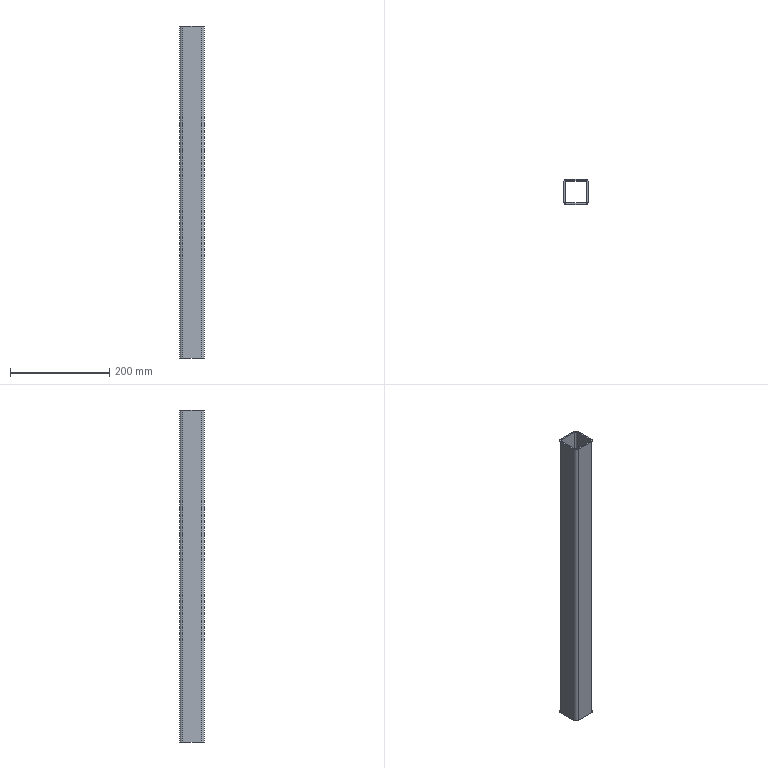Part | SolidWorks | 1 solid | 18 faces | box 50 x 50 x 670 mm | volume 362351 mm3 | plane 10 | cylinder 8 | commonest cylinder face diameters 6 x4 12 x4
STEP:
#1=CARTESIAN_POINT('',(19.,25.,335.));
#2=VERTEX_POINT('',#1);
#3=CARTESIAN_POINT('',(25.,19.,335.));
#4=VERTEX_POINT('',#3);
#5=CARTESIAN_POINT('',(19.,19.,335.));
#6=DIRECTION('',(0.,0.,-1.));
#7=DIRECTION('',(-1.,0.,0.));
#8=AXIS2_PLACEMENT_3D('',#5,#6,#7);
#9=CIRCLE('',#8,6.);
#10=EDGE_CURVE('',#2,#4,#9,.T.);
#11=ORIENTED_EDGE('',*,*,#10,.T.);
#12=CARTESIAN_POINT('',(25.,19.,-335.));
#13=VERTEX_POINT('',#12);
#14=CARTESIAN_POINT('',(25.,19.,-335.));
#15=DIRECTION('',(0.,0.,1.));
#16=VECTOR('',#15,1000.);
#17=LINE('',#14,#16);
#18=EDGE_CURVE('',#13,#4,#17,.T.);
#19=ORIENTED_EDGE('',*,*,#18,.F.);
#20=CARTESIAN_POINT('',(19.,25.,-335.));
#21=VERTEX_POINT('',#20);
#22=CARTESIAN_POINT('',(19.,19.,-335.));
#23=DIRECTION('',(0.,0.,-1.));
#24=DIRECTION('',(-1.,0.,0.));
#25=AXIS2_PLACEMENT_3D('',#22,#23,#24);
#26=CIRCLE('',#25,6.);
#27=EDGE_CURVE('',#21,#13,#26,.T.);
#28=ORIENTED_EDGE('',*,*,#27,.F.);
#29=CARTESIAN_POINT('',(19.,25.,-335.));
#30=DIRECTION('',(0.,0.,1.));
#31=VECTOR('',#30,1000.);
#32=LINE('',#29,#31);
#33=EDGE_CURVE('',#21,#2,#32,.T.);
#34=ORIENTED_EDGE('',*,*,#33,.T.);
#35=EDGE_LOOP('',(#11,#19,#28,#34));
#36=FACE_OUTER_BOUND('',#35,.T.);
#37=CARTESIAN_POINT('',(19.,19.,-335.));
#38=DIRECTION('',(0.,0.,1.));
#39=DIRECTION('',(1.,0.,0.));
#40=AXIS2_PLACEMENT_3D('',#37,#38,#39);
#41=CYLINDRICAL_SURFACE('',#40,6.);
#42=ADVANCED_FACE('',(#36),#41,.T.);
#43=CARTESIAN_POINT('',(25.,-19.,335.));
#44=VERTEX_POINT('',#43);
#45=CARTESIAN_POINT('',(25.,19.,335.));
#46=DIRECTION('',(0.,-1.,0.));
#47=VECTOR('',#46,1000.);
#48=LINE('',#45,#47);
#49=EDGE_CURVE('',#4,#44,#48,.T.);
#50=ORIENTED_EDGE('',*,*,#49,.T.);
#51=CARTESIAN_POINT('',(25.,-19.,-335.));
#52=VERTEX_POINT('',#51);
#53=CARTESIAN_POINT('',(25.,-19.,-335.));
#54=DIRECTION('',(0.,0.,1.));
#55=VECTOR('',#54,1000.);
#56=LINE('',#53,#55);
#57=EDGE_CURVE('',#52,#44,#56,.T.);
#58=ORIENTED_EDGE('',*,*,#57,.F.);
#59=CARTESIAN_POINT('',(25.,19.,-335.));
#60=DIRECTION('',(0.,-1.,0.));
#61=VECTOR('',#60,1000.);
#62=LINE('',#59,#61);
#63=EDGE_CURVE('',#13,#52,#62,.T.);
#64=ORIENTED_EDGE('',*,*,#63,.F.);
#65=ORIENTED_EDGE('',*,*,#18,.T.);
#66=EDGE_LOOP('',(#50,#58,#64,#65));
#67=FACE_OUTER_BOUND('',#66,.T.);
#68=CARTESIAN_POINT('',(25.,19.,-335.));
#69=DIRECTION('',(-1.,0.,0.));
#70=DIRECTION('',(0.,0.,1.));
#71=AXIS2_PLACEMENT_3D('',#68,#69,#70);
#72=PLANE('',#71);
#73=ADVANCED_FACE('',(#67),#72,.F.);
#74=CARTESIAN_POINT('',(19.,-25.,335.));
#75=VERTEX_POINT('',#74);
#76=CARTESIAN_POINT('',(19.,-19.,335.));
#77=DIRECTION('',(0.,0.,-1.));
#78=DIRECTION('',(-1.,0.,0.));
#79=AXIS2_PLACEMENT_3D('',#76,#77,#78);
#80=CIRCLE('',#79,6.);
#81=EDGE_CURVE('',#44,#75,#80,.T.);
#82=ORIENTED_EDGE('',*,*,#81,.T.);
#83=CARTESIAN_POINT('',(19.,-25.,-335.));
#84=VERTEX_POINT('',#83);
#85=CARTESIAN_POINT('',(19.,-25.,-335.));
#86=DIRECTION('',(0.,0.,1.));
#87=VECTOR('',#86,1000.);
#88=LINE('',#85,#87);
#89=EDGE_CURVE('',#84,#75,#88,.T.);
#90=ORIENTED_EDGE('',*,*,#89,.F.);
#91=CARTESIAN_POINT('',(19.,-19.,-335.));
#92=DIRECTION('',(0.,0.,-1.));
#93=DIRECTION('',(-1.,0.,0.));
#94=AXIS2_PLACEMENT_3D('',#91,#92,#93);
#95=CIRCLE('',#94,6.);
#96=EDGE_CURVE('',#52,#84,#95,.T.);
#97=ORIENTED_EDGE('',*,*,#96,.F.);
#98=ORIENTED_EDGE('',*,*,#57,.T.);
#99=EDGE_LOOP('',(#82,#90,#97,#98));
#100=FACE_OUTER_BOUND('',#99,.T.);
#101=CARTESIAN_POINT('',(19.,-19.,-335.));
#102=DIRECTION('',(0.,0.,1.));
#103=DIRECTION('',(1.,0.,0.));
#104=AXIS2_PLACEMENT_3D('',#101,#102,#103);
#105=CYLINDRICAL_SURFACE('',#104,6.);
#106=ADVANCED_FACE('',(#100),#105,.T.);
#107=CARTESIAN_POINT('',(-19.,-25.,335.));
#108=VERTEX_POINT('',#107);
#109=CARTESIAN_POINT('',(-19.,-25.,335.));
#110=DIRECTION('',(-1.,0.,0.));
#111=VECTOR('',#110,1000.);
#112=LINE('',#109,#111);
#113=EDGE_CURVE('',#75,#108,#112,.T.);
#114=ORIENTED_EDGE('',*,*,#113,.T.);
#115=CARTESIAN_POINT('',(-19.,-25.,-335.));
#116=VERTEX_POINT('',#115);
#117=CARTESIAN_POINT('',(-19.,-25.,-335.));
#118=DIRECTION('',(0.,0.,1.));
#119=VECTOR('',#118,1000.);
#120=LINE('',#117,#119);
#121=EDGE_CURVE('',#116,#108,#120,.T.);
#122=ORIENTED_EDGE('',*,*,#121,.F.);
#123=CARTESIAN_POINT('',(-19.,-25.,-335.));
#124=DIRECTION('',(-1.,0.,0.));
#125=VECTOR('',#124,1000.);
#126=LINE('',#123,#125);
#127=EDGE_CURVE('',#84,#116,#126,.T.);
#128=ORIENTED_EDGE('',*,*,#127,.F.);
#129=ORIENTED_EDGE('',*,*,#89,.T.);
#130=EDGE_LOOP('',(#114,#122,#128,#129));
#131=FACE_OUTER_BOUND('',#130,.T.);
#132=CARTESIAN_POINT('',(-19.,-25.,-335.));
#133=DIRECTION('',(0.,1.,0.));
#134=DIRECTION('',(0.,0.,1.));
#135=AXIS2_PLACEMENT_3D('',#132,#133,#134);
#136=PLANE('',#135);
#137=ADVANCED_FACE('',(#131),#136,.F.);
#138=CARTESIAN_POINT('',(-25.,-19.,335.));
#139=VERTEX_POINT('',#138);
#140=CARTESIAN_POINT('',(-19.,-19.,335.));
#141=DIRECTION('',(0.,0.,-1.));
#142=DIRECTION('',(-1.,0.,0.));
#143=AXIS2_PLACEMENT_3D('',#140,#141,#142);
#144=CIRCLE('',#143,6.);
#145=EDGE_CURVE('',#108,#139,#144,.T.);
#146=ORIENTED_EDGE('',*,*,#145,.T.);
#147=CARTESIAN_POINT('',(-25.,-19.,-335.));
#148=VERTEX_POINT('',#147);
#149=CARTESIAN_POINT('',(-25.,-19.,-335.));
#150=DIRECTION('',(0.,0.,1.));
#151=VECTOR('',#150,1000.);
#152=LINE('',#149,#151);
#153=EDGE_CURVE('',#148,#139,#152,.T.);
#154=ORIENTED_EDGE('',*,*,#153,.F.);
#155=CARTESIAN_POINT('',(-19.,-19.,-335.));
#156=DIRECTION('',(0.,0.,-1.));
#157=DIRECTION('',(-1.,0.,0.));
#158=AXIS2_PLACEMENT_3D('',#155,#156,#157);
#159=CIRCLE('',#158,6.);
#160=EDGE_CURVE('',#116,#148,#159,.T.);
#161=ORIENTED_EDGE('',*,*,#160,.F.);
#162=ORIENTED_EDGE('',*,*,#121,.T.);
#163=EDGE_LOOP('',(#146,#154,#161,#162));
#164=FACE_OUTER_BOUND('',#163,.T.);
#165=CARTESIAN_POINT('',(-19.,-19.,-335.));
#166=DIRECTION('',(0.,0.,1.));
#167=DIRECTION('',(1.,0.,0.));
#168=AXIS2_PLACEMENT_3D('',#165,#166,#167);
#169=CYLINDRICAL_SURFACE('',#168,6.);
#170=ADVANCED_FACE('',(#164),#169,.T.);
#171=CARTESIAN_POINT('',(-25.,19.,335.));
#172=VERTEX_POINT('',#171);
#173=CARTESIAN_POINT('',(-25.,-19.,335.));
#174=DIRECTION('',(0.,1.,0.));
#175=VECTOR('',#174,1000.);
#176=LINE('',#173,#175);
#177=EDGE_CURVE('',#139,#172,#176,.T.);
#178=ORIENTED_EDGE('',*,*,#177,.T.);
#179=CARTESIAN_POINT('',(-25.,19.,-335.));
#180=VERTEX_POINT('',#179);
#181=CARTESIAN_POINT('',(-25.,19.,-335.));
#182=DIRECTION('',(0.,0.,1.));
#183=VECTOR('',#182,1000.);
#184=LINE('',#181,#183);
#185=EDGE_CURVE('',#180,#172,#184,.T.);
#186=ORIENTED_EDGE('',*,*,#185,.F.);
#187=CARTESIAN_POINT('',(-25.,-19.,-335.));
#188=DIRECTION('',(0.,1.,0.));
#189=VECTOR('',#188,1000.);
#190=LINE('',#187,#189);
#191=EDGE_CURVE('',#148,#180,#190,.T.);
#192=ORIENTED_EDGE('',*,*,#191,.F.);
#193=ORIENTED_EDGE('',*,*,#153,.T.);
#194=EDGE_LOOP('',(#178,#186,#192,#193));
#195=FACE_OUTER_BOUND('',#194,.T.);
#196=CARTESIAN_POINT('',(-25.,-19.,-335.));
#197=DIRECTION('',(1.,0.,0.));
#198=DIRECTION('',(0.,0.,-1.));
#199=AXIS2_PLACEMENT_3D('',#196,#197,#198);
#200=PLANE('',#199);
#201=ADVANCED_FACE('',(#195),#200,.F.);
#202=CARTESIAN_POINT('',(-19.,25.,335.));
#203=VERTEX_POINT('',#202);
#204=CARTESIAN_POINT('',(-19.,19.,335.));
#205=DIRECTION('',(0.,0.,-1.));
#206=DIRECTION('',(-1.,0.,0.));
#207=AXIS2_PLACEMENT_3D('',#204,#205,#206);
#208=CIRCLE('',#207,6.);
#209=EDGE_CURVE('',#172,#203,#208,.T.);
#210=ORIENTED_EDGE('',*,*,#209,.T.);
#211=CARTESIAN_POINT('',(-19.,25.,-335.));
#212=VERTEX_POINT('',#211);
#213=CARTESIAN_POINT('',(-19.,25.,-335.));
#214=DIRECTION('',(0.,0.,1.));
#215=VECTOR('',#214,1000.);
#216=LINE('',#213,#215);
#217=EDGE_CURVE('',#212,#203,#216,.T.);
#218=ORIENTED_EDGE('',*,*,#217,.F.);
#219=CARTESIAN_POINT('',(-19.,19.,-335.));
#220=DIRECTION('',(0.,0.,-1.));
#221=DIRECTION('',(-1.,0.,0.));
#222=AXIS2_PLACEMENT_3D('',#219,#220,#221);
#223=CIRCLE('',#222,6.);
#224=EDGE_CURVE('',#180,#212,#223,.T.);
#225=ORIENTED_EDGE('',*,*,#224,.F.);
#226=ORIENTED_EDGE('',*,*,#185,.T.);
#227=EDGE_LOOP('',(#210,#218,#225,#226));
#228=FACE_OUTER_BOUND('',#227,.T.);
#229=CARTESIAN_POINT('',(-19.,19.,-335.));
#230=DIRECTION('',(0.,0.,1.));
#231=DIRECTION('',(1.,0.,0.));
#232=AXIS2_PLACEMENT_3D('',#229,#230,#231);
#233=CYLINDRICAL_SURFACE('',#232,6.);
#234=ADVANCED_FACE('',(#228),#233,.T.);
#235=CARTESIAN_POINT('',(22.,-19.,335.));
#236=VERTEX_POINT('',#235);
#237=CARTESIAN_POINT('',(19.,-22.,335.));
#238=VERTEX_POINT('',#237);
#239=CARTESIAN_POINT('',(19.,-19.,335.));
#240=DIRECTION('',(0.,0.,-1.));
#241=DIRECTION('',(-1.,0.,0.));
#242=AXIS2_PLACEMENT_3D('',#239,#240,#241);
#243=CIRCLE('',#242,3.);
#244=EDGE_CURVE('',#236,#238,#243,.T.);
#245=ORIENTED_EDGE('',*,*,#244,.F.);
#246=CARTESIAN_POINT('',(22.,-19.,-335.));
#247=VERTEX_POINT('',#246);
#248=CARTESIAN_POINT('',(22.,-19.,-335.));
#249=DIRECTION('',(0.,0.,1.));
#250=VECTOR('',#249,1000.);
#251=LINE('',#248,#250);
#252=EDGE_CURVE('',#247,#236,#251,.T.);
#253=ORIENTED_EDGE('',*,*,#252,.F.);
#254=CARTESIAN_POINT('',(19.,-22.,-335.));
#255=VERTEX_POINT('',#254);
#256=CARTESIAN_POINT('',(19.,-19.,-335.));
#257=DIRECTION('',(0.,0.,-1.));
#258=DIRECTION('',(-1.,0.,0.));
#259=AXIS2_PLACEMENT_3D('',#256,#257,#258);
#260=CIRCLE('',#259,3.);
#261=EDGE_CURVE('',#247,#255,#260,.T.);
#262=ORIENTED_EDGE('',*,*,#261,.T.);
#263=CARTESIAN_POINT('',(19.,-22.,-335.));
#264=DIRECTION('',(0.,0.,1.));
#265=VECTOR('',#264,1000.);
#266=LINE('',#263,#265);
#267=EDGE_CURVE('',#255,#238,#266,.T.);
#268=ORIENTED_EDGE('',*,*,#267,.T.);
#269=EDGE_LOOP('',(#245,#253,#262,#268));
#270=FACE_OUTER_BOUND('',#269,.T.);
#271=CARTESIAN_POINT('',(19.,-19.,-335.));
#272=DIRECTION('',(0.,0.,1.));
#273=DIRECTION('',(1.,0.,0.));
#274=AXIS2_PLACEMENT_3D('',#271,#272,#273);
#275=CYLINDRICAL_SURFACE('',#274,3.);
#276=ADVANCED_FACE('',(#270),#275,.F.);
#277=CARTESIAN_POINT('',(22.,19.,335.));
#278=VERTEX_POINT('',#277);
#279=CARTESIAN_POINT('',(22.,19.,335.));
#280=DIRECTION('',(0.,-1.,0.));
#281=VECTOR('',#280,1000.);
#282=LINE('',#279,#281);
#283=EDGE_CURVE('',#278,#236,#282,.T.);
#284=ORIENTED_EDGE('',*,*,#283,.F.);
#285=CARTESIAN_POINT('',(22.,19.,-335.));
#286=VERTEX_POINT('',#285);
#287=CARTESIAN_POINT('',(22.,19.,-335.));
#288=DIRECTION('',(0.,0.,1.));
#289=VECTOR('',#288,1000.);
#290=LINE('',#287,#289);
#291=EDGE_CURVE('',#286,#278,#290,.T.);
#292=ORIENTED_EDGE('',*,*,#291,.F.);
#293=CARTESIAN_POINT('',(22.,19.,-335.));
#294=DIRECTION('',(0.,-1.,0.));
#295=VECTOR('',#294,1000.);
#296=LINE('',#293,#295);
#297=EDGE_CURVE('',#286,#247,#296,.T.);
#298=ORIENTED_EDGE('',*,*,#297,.T.);
#299=ORIENTED_EDGE('',*,*,#252,.T.);
#300=EDGE_LOOP('',(#284,#292,#298,#299));
#301=FACE_OUTER_BOUND('',#300,.T.);
#302=CARTESIAN_POINT('',(22.,19.,-335.));
#303=DIRECTION('',(-1.,0.,0.));
#304=DIRECTION('',(0.,0.,1.));
#305=AXIS2_PLACEMENT_3D('',#302,#303,#304);
#306=PLANE('',#305);
#307=ADVANCED_FACE('',(#301),#306,.T.);
#308=CARTESIAN_POINT('',(19.,22.,335.));
#309=VERTEX_POINT('',#308);
#310=CARTESIAN_POINT('',(19.,19.,335.));
#311=DIRECTION('',(0.,0.,-1.));
#312=DIRECTION('',(-1.,0.,0.));
#313=AXIS2_PLACEMENT_3D('',#310,#311,#312);
#314=CIRCLE('',#313,3.);
#315=EDGE_CURVE('',#309,#278,#314,.T.);
#316=ORIENTED_EDGE('',*,*,#315,.F.);
#317=CARTESIAN_POINT('',(19.,22.,-335.));
#318=VERTEX_POINT('',#317);
#319=CARTESIAN_POINT('',(19.,22.,-335.));
#320=DIRECTION('',(0.,0.,1.));
#321=VECTOR('',#320,1000.);
#322=LINE('',#319,#321);
#323=EDGE_CURVE('',#318,#309,#322,.T.);
#324=ORIENTED_EDGE('',*,*,#323,.F.);
#325=CARTESIAN_POINT('',(19.,19.,-335.));
#326=DIRECTION('',(0.,0.,-1.));
#327=DIRECTION('',(-1.,0.,0.));
#328=AXIS2_PLACEMENT_3D('',#325,#326,#327);
#329=CIRCLE('',#328,3.);
#330=EDGE_CURVE('',#318,#286,#329,.T.);
#331=ORIENTED_EDGE('',*,*,#330,.T.);
#332=ORIENTED_EDGE('',*,*,#291,.T.);
#333=EDGE_LOOP('',(#316,#324,#331,#332));
#334=FACE_OUTER_BOUND('',#333,.T.);
#335=CARTESIAN_POINT('',(19.,19.,-335.));
#336=DIRECTION('',(0.,0.,1.));
#337=DIRECTION('',(1.,0.,0.));
#338=AXIS2_PLACEMENT_3D('',#335,#336,#337);
#339=CYLINDRICAL_SURFACE('',#338,3.);
#340=ADVANCED_FACE('',(#334),#339,.F.);
#341=CARTESIAN_POINT('',(-19.,22.,335.));
#342=VERTEX_POINT('',#341);
#343=CARTESIAN_POINT('',(19.,22.,335.));
#344=DIRECTION('',(1.,0.,0.));
#345=VECTOR('',#344,1000.);
#346=LINE('',#343,#345);
#347=EDGE_CURVE('',#342,#309,#346,.T.);
#348=ORIENTED_EDGE('',*,*,#347,.F.);
#349=CARTESIAN_POINT('',(-19.,22.,-335.));
#350=VERTEX_POINT('',#349);
#351=CARTESIAN_POINT('',(-19.,22.,-335.));
#352=DIRECTION('',(0.,0.,1.));
#353=VECTOR('',#352,1000.);
#354=LINE('',#351,#353);
#355=EDGE_CURVE('',#350,#342,#354,.T.);
#356=ORIENTED_EDGE('',*,*,#355,.F.);
#357=CARTESIAN_POINT('',(19.,22.,-335.));
#358=DIRECTION('',(1.,0.,0.));
#359=VECTOR('',#358,1000.);
#360=LINE('',#357,#359);
#361=EDGE_CURVE('',#350,#318,#360,.T.);
#362=ORIENTED_EDGE('',*,*,#361,.T.);
#363=ORIENTED_EDGE('',*,*,#323,.T.);
#364=EDGE_LOOP('',(#348,#356,#362,#363));
#365=FACE_OUTER_BOUND('',#364,.T.);
#366=CARTESIAN_POINT('',(19.,22.,-335.));
#367=DIRECTION('',(0.,-1.,0.));
#368=DIRECTION('',(0.,0.,-1.));
#369=AXIS2_PLACEMENT_3D('',#366,#367,#368);
#370=PLANE('',#369);
#371=ADVANCED_FACE('',(#365),#370,.T.);
#372=CARTESIAN_POINT('',(-22.,19.,335.));
#373=VERTEX_POINT('',#372);
#374=CARTESIAN_POINT('',(-19.,19.,335.));
#375=DIRECTION('',(0.,0.,-1.));
#376=DIRECTION('',(-1.,0.,0.));
#377=AXIS2_PLACEMENT_3D('',#374,#375,#376);
#378=CIRCLE('',#377,3.);
#379=EDGE_CURVE('',#373,#342,#378,.T.);
#380=ORIENTED_EDGE('',*,*,#379,.F.);
#381=CARTESIAN_POINT('',(-22.,19.,-335.));
#382=VERTEX_POINT('',#381);
#383=CARTESIAN_POINT('',(-22.,19.,-335.));
#384=DIRECTION('',(0.,0.,1.));
#385=VECTOR('',#384,1000.);
#386=LINE('',#383,#385);
#387=EDGE_CURVE('',#382,#373,#386,.T.);
#388=ORIENTED_EDGE('',*,*,#387,.F.);
#389=CARTESIAN_POINT('',(-19.,19.,-335.));
#390=DIRECTION('',(0.,0.,-1.));
#391=DIRECTION('',(-1.,0.,0.));
#392=AXIS2_PLACEMENT_3D('',#389,#390,#391);
#393=CIRCLE('',#392,3.);
#394=EDGE_CURVE('',#382,#350,#393,.T.);
#395=ORIENTED_EDGE('',*,*,#394,.T.);
#396=ORIENTED_EDGE('',*,*,#355,.T.);
#397=EDGE_LOOP('',(#380,#388,#395,#396));
#398=FACE_OUTER_BOUND('',#397,.T.);
#399=CARTESIAN_POINT('',(-19.,19.,-335.));
#400=DIRECTION('',(0.,0.,1.));
#401=DIRECTION('',(1.,0.,0.));
#402=AXIS2_PLACEMENT_3D('',#399,#400,#401);
#403=CYLINDRICAL_SURFACE('',#402,3.);
#404=ADVANCED_FACE('',(#398),#403,.F.);
#405=CARTESIAN_POINT('',(-22.,-19.,335.));
#406=VERTEX_POINT('',#405);
#407=CARTESIAN_POINT('',(-22.,-19.,335.));
#408=DIRECTION('',(0.,1.,0.));
#409=VECTOR('',#408,1000.);
#410=LINE('',#407,#409);
#411=EDGE_CURVE('',#406,#373,#410,.T.);
#412=ORIENTED_EDGE('',*,*,#411,.F.);
#413=CARTESIAN_POINT('',(-22.,-19.,-335.));
#414=VERTEX_POINT('',#413);
#415=CARTESIAN_POINT('',(-22.,-19.,-335.));
#416=DIRECTION('',(0.,0.,1.));
#417=VECTOR('',#416,1000.);
#418=LINE('',#415,#417);
#419=EDGE_CURVE('',#414,#406,#418,.T.);
#420=ORIENTED_EDGE('',*,*,#419,.F.);
#421=CARTESIAN_POINT('',(-22.,-19.,-335.));
#422=DIRECTION('',(0.,1.,0.));
#423=VECTOR('',#422,1000.);
#424=LINE('',#421,#423);
#425=EDGE_CURVE('',#414,#382,#424,.T.);
#426=ORIENTED_EDGE('',*,*,#425,.T.);
#427=ORIENTED_EDGE('',*,*,#387,.T.);
#428=EDGE_LOOP('',(#412,#420,#426,#427));
#429=FACE_OUTER_BOUND('',#428,.T.);
#430=CARTESIAN_POINT('',(-22.,-19.,-335.));
#431=DIRECTION('',(1.,0.,0.));
#432=DIRECTION('',(0.,0.,-1.));
#433=AXIS2_PLACEMENT_3D('',#430,#431,#432);
#434=PLANE('',#433);
#435=ADVANCED_FACE('',(#429),#434,.T.);
#436=CARTESIAN_POINT('',(-19.,-22.,335.));
#437=VERTEX_POINT('',#436);
#438=CARTESIAN_POINT('',(-19.,-19.,335.));
#439=DIRECTION('',(0.,0.,-1.));
#440=DIRECTION('',(-1.,0.,0.));
#441=AXIS2_PLACEMENT_3D('',#438,#439,#440);
#442=CIRCLE('',#441,3.);
#443=EDGE_CURVE('',#437,#406,#442,.T.);
#444=ORIENTED_EDGE('',*,*,#443,.F.);
#445=CARTESIAN_POINT('',(-19.,-22.,-335.));
#446=VERTEX_POINT('',#445);
#447=CARTESIAN_POINT('',(-19.,-22.,-335.));
#448=DIRECTION('',(0.,0.,1.));
#449=VECTOR('',#448,1000.);
#450=LINE('',#447,#449);
#451=EDGE_CURVE('',#446,#437,#450,.T.);
#452=ORIENTED_EDGE('',*,*,#451,.F.);
#453=CARTESIAN_POINT('',(-19.,-19.,-335.));
#454=DIRECTION('',(0.,0.,-1.));
#455=DIRECTION('',(-1.,0.,0.));
#456=AXIS2_PLACEMENT_3D('',#453,#454,#455);
#457=CIRCLE('',#456,3.);
#458=EDGE_CURVE('',#446,#414,#457,.T.);
#459=ORIENTED_EDGE('',*,*,#458,.T.);
#460=ORIENTED_EDGE('',*,*,#419,.T.);
#461=EDGE_LOOP('',(#444,#452,#459,#460));
#462=FACE_OUTER_BOUND('',#461,.T.);
#463=CARTESIAN_POINT('',(-19.,-19.,-335.));
#464=DIRECTION('',(0.,0.,1.));
#465=DIRECTION('',(1.,0.,0.));
#466=AXIS2_PLACEMENT_3D('',#463,#464,#465);
#467=CYLINDRICAL_SURFACE('',#466,3.);
#468=ADVANCED_FACE('',(#462),#467,.F.);
#469=CARTESIAN_POINT('',(-19.,-22.,335.));
#470=DIRECTION('',(-1.,0.,0.));
#471=VECTOR('',#470,1000.);
#472=LINE('',#469,#471);
#473=EDGE_CURVE('',#238,#437,#472,.T.);
#474=ORIENTED_EDGE('',*,*,#473,.F.);
#475=ORIENTED_EDGE('',*,*,#267,.F.);
#476=CARTESIAN_POINT('',(-19.,-22.,-335.));
#477=DIRECTION('',(-1.,0.,0.));
#478=VECTOR('',#477,1000.);
#479=LINE('',#476,#478);
#480=EDGE_CURVE('',#255,#446,#479,.T.);
#481=ORIENTED_EDGE('',*,*,#480,.T.);
#482=ORIENTED_EDGE('',*,*,#451,.T.);
#483=EDGE_LOOP('',(#474,#475,#481,#482));
#484=FACE_OUTER_BOUND('',#483,.T.);
#485=CARTESIAN_POINT('',(-19.,-22.,-335.));
#486=DIRECTION('',(0.,1.,0.));
#487=DIRECTION('',(0.,0.,1.));
#488=AXIS2_PLACEMENT_3D('',#485,#486,#487);
#489=PLANE('',#488);
#490=ADVANCED_FACE('',(#484),#489,.T.);
#491=CARTESIAN_POINT('',(19.,25.,335.));
#492=DIRECTION('',(1.,0.,0.));
#493=VECTOR('',#492,1000.);
#494=LINE('',#491,#493);
#495=EDGE_CURVE('',#203,#2,#494,.T.);
#496=ORIENTED_EDGE('',*,*,#495,.T.);
#497=ORIENTED_EDGE('',*,*,#33,.F.);
#498=CARTESIAN_POINT('',(19.,25.,-335.));
#499=DIRECTION('',(1.,0.,0.));
#500=VECTOR('',#499,1000.);
#501=LINE('',#498,#500);
#502=EDGE_CURVE('',#212,#21,#501,.T.);
#503=ORIENTED_EDGE('',*,*,#502,.F.);
#504=ORIENTED_EDGE('',*,*,#217,.T.);
#505=EDGE_LOOP('',(#496,#497,#503,#504));
#506=FACE_OUTER_BOUND('',#505,.T.);
#507=CARTESIAN_POINT('',(19.,25.,-335.));
#508=DIRECTION('',(0.,-1.,0.));
#509=DIRECTION('',(0.,0.,-1.));
#510=AXIS2_PLACEMENT_3D('',#507,#508,#509);
#511=PLANE('',#510);
#512=ADVANCED_FACE('',(#506),#511,.F.);
#513=ORIENTED_EDGE('',*,*,#261,.F.);
#514=ORIENTED_EDGE('',*,*,#297,.F.);
#515=ORIENTED_EDGE('',*,*,#330,.F.);
#516=ORIENTED_EDGE('',*,*,#361,.F.);
#517=ORIENTED_EDGE('',*,*,#394,.F.);
#518=ORIENTED_EDGE('',*,*,#425,.F.);
#519=ORIENTED_EDGE('',*,*,#458,.F.);
#520=ORIENTED_EDGE('',*,*,#480,.F.);
#521=EDGE_LOOP('',(#513,#514,#515,#516,#517,#518,#519,#520));
#522=FACE_BOUND('',#521,.T.);
#523=ORIENTED_EDGE('',*,*,#27,.T.);
#524=ORIENTED_EDGE('',*,*,#63,.T.);
#525=ORIENTED_EDGE('',*,*,#96,.T.);
#526=ORIENTED_EDGE('',*,*,#127,.T.);
#527=ORIENTED_EDGE('',*,*,#160,.T.);
#528=ORIENTED_EDGE('',*,*,#191,.T.);
#529=ORIENTED_EDGE('',*,*,#224,.T.);
#530=ORIENTED_EDGE('',*,*,#502,.T.);
#531=EDGE_LOOP('',(#523,#524,#525,#526,#527,#528,#529,#530));
#532=FACE_OUTER_BOUND('',#531,.T.);
#533=CARTESIAN_POINT('',(19.,19.,-335.));
#534=DIRECTION('',(0.,0.,-1.));
#535=DIRECTION('',(-1.,0.,0.));
#536=AXIS2_PLACEMENT_3D('',#533,#534,#535);
#537=PLANE('',#536);
#538=ADVANCED_FACE('',(#522,#532),#537,.T.);
#539=ORIENTED_EDGE('',*,*,#244,.T.);
#540=ORIENTED_EDGE('',*,*,#473,.T.);
#541=ORIENTED_EDGE('',*,*,#443,.T.);
#542=ORIENTED_EDGE('',*,*,#411,.T.);
#543=ORIENTED_EDGE('',*,*,#379,.T.);
#544=ORIENTED_EDGE('',*,*,#347,.T.);
#545=ORIENTED_EDGE('',*,*,#315,.T.);
#546=ORIENTED_EDGE('',*,*,#283,.T.);
#547=EDGE_LOOP('',(#539,#540,#541,#542,#543,#544,#545,#546));
#548=FACE_BOUND('',#547,.T.);
#549=ORIENTED_EDGE('',*,*,#10,.F.);
#550=ORIENTED_EDGE('',*,*,#495,.F.);
#551=ORIENTED_EDGE('',*,*,#209,.F.);
#552=ORIENTED_EDGE('',*,*,#177,.F.);
#553=ORIENTED_EDGE('',*,*,#145,.F.);
#554=ORIENTED_EDGE('',*,*,#113,.F.);
#555=ORIENTED_EDGE('',*,*,#81,.F.);
#556=ORIENTED_EDGE('',*,*,#49,.F.);
#557=EDGE_LOOP('',(#549,#550,#551,#552,#553,#554,#555,#556));
#558=FACE_OUTER_BOUND('',#557,.T.);
#559=CARTESIAN_POINT('',(19.,19.,335.));
#560=DIRECTION('',(0.,0.,-1.));
#561=DIRECTION('',(-1.,0.,0.));
#562=AXIS2_PLACEMENT_3D('',#559,#560,#561);
#563=PLANE('',#562);
#564=ADVANCED_FACE('',(#548,#558),#563,.F.);
#565=CLOSED_SHELL('',(#42,#73,#106,#137,#170,#201,#234,#276,#307,#340,#371,#404,#435,#468,#490,#512,#538,#564));
#566=MANIFOLD_SOLID_BREP('',#565);
#567=CARTESIAN_POINT('',(0.,0.,0.));
#568=DIRECTION('',(0.,0.,1.));
#569=DIRECTION('',(1.,0.,0.));
#570=AXIS2_PLACEMENT_3D('',#567,#568,#569);
#571=(LENGTH_UNIT()NAMED_UNIT(*)SI_UNIT(.MILLI.,.METRE.));
#572=UNCERTAINTY_MEASURE_WITH_UNIT(LENGTH_MEASURE(0.00001),#571,'','');
#573=(NAMED_UNIT(*)PLANE_ANGLE_UNIT()SI_UNIT($,.RADIAN.));
#574=(NAMED_UNIT(*)SI_UNIT($,.STERADIAN.)SOLID_ANGLE_UNIT());
#575=(GEOMETRIC_REPRESENTATION_CONTEXT(3)GLOBAL_UNCERTAINTY_ASSIGNED_CONTEXT((#572))GLOBAL_UNIT_ASSIGNED_CONTEXT((#571,#573,#574))REPRESENTATION_CONTEXT('',''));
#576=ADVANCED_BREP_SHAPE_REPRESENTATION('',(#566,#570),#575);